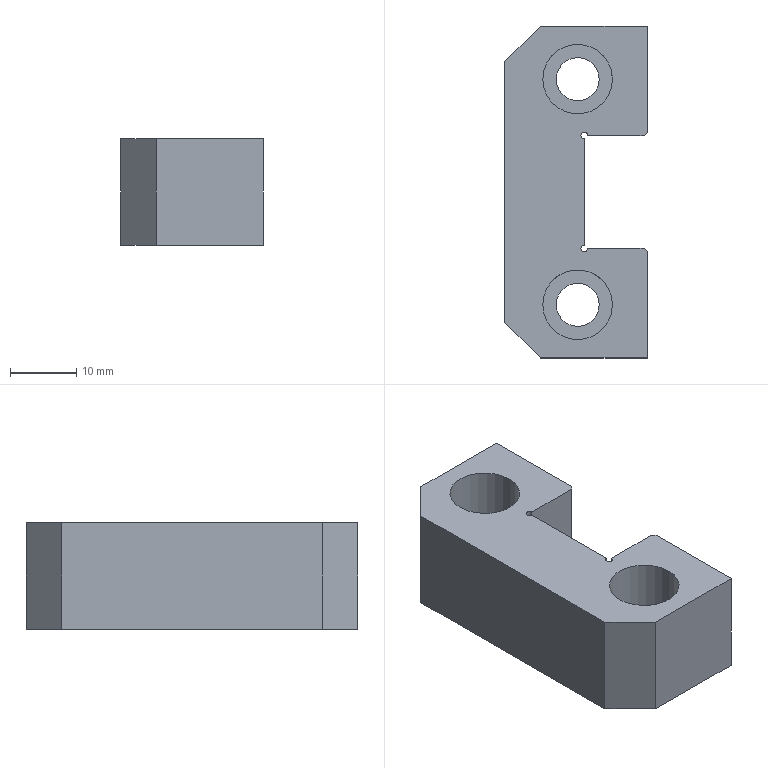Part | STEP file | 1_1 | 1 solid | 28 faces | box 21.5 x 50 x 16 mm | volume 12210 mm3 | plane 16 | cylinder 12 | commonest cylinder face diameters 1 x4 6.5 x4 10.5 x4